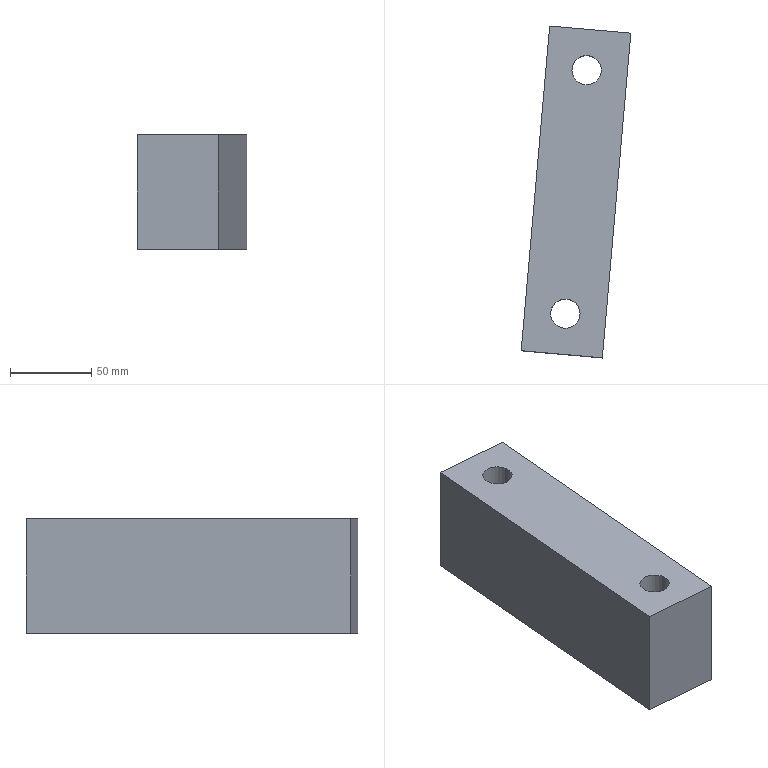Part | NX | features solid 2 | 1 solid | 8 faces | box 67.241 x 203.597 x 70 mm | volume 664374 mm3 | plane 6 | cylinder 2 | commonest cylinder face diameters 18 x2
STEP:
#1=CARTESIAN_POINT('',(193.983,-191.852,-70.));
#2=VERTEX_POINT('',#1);
#3=CARTESIAN_POINT('',(184.983,-191.852,-70.));
#4=DIRECTION('',(0.,0.,1.));
#5=DIRECTION('',(1.,0.,0.));
#6=AXIS2_PLACEMENT_3D('',#3,#4,#5);
#7=CIRCLE('',#6,9.);
#8=EDGE_CURVE('',#2,#2,#7,.T.);
#9=ORIENTED_EDGE('',*,*,#8,.F.);
#10=EDGE_LOOP('',(#9));
#11=FACE_BOUND('',#10,.T.);
#12=CARTESIAN_POINT('',(207.056,-42.423,-70.));
#13=VERTEX_POINT('',#12);
#14=CARTESIAN_POINT('',(198.056,-42.423,-70.));
#15=DIRECTION('',(0.,0.,1.));
#16=DIRECTION('',(1.,0.,0.));
#17=AXIS2_PLACEMENT_3D('',#14,#15,#16);
#18=CIRCLE('',#17,9.);
#19=EDGE_CURVE('',#13,#13,#18,.T.);
#20=ORIENTED_EDGE('',*,*,#19,.F.);
#21=EDGE_LOOP('',(#20));
#22=FACE_BOUND('',#21,.T.);
#23=CARTESIAN_POINT('',(175.33,-15.339,-70.));
#24=VERTEX_POINT('',#23);
#25=CARTESIAN_POINT('',(225.14,-19.697,-70.));
#26=VERTEX_POINT('',#25);
#27=CARTESIAN_POINT('',(175.33,-15.339,-70.));
#28=DIRECTION('',(0.9962,-0.08716,0.));
#29=VECTOR('',#28,1000.);
#30=LINE('',#27,#29);
#31=EDGE_CURVE('',#24,#26,#30,.T.);
#32=ORIENTED_EDGE('',*,*,#31,.F.);
#33=CARTESIAN_POINT('',(157.899,-214.578,-70.));
#34=VERTEX_POINT('',#33);
#35=CARTESIAN_POINT('',(162.257,-164.769,-70.));
#36=DIRECTION('',(0.08716,0.9962,0.));
#37=VECTOR('',#36,1000.);
#38=LINE('',#35,#37);
#39=EDGE_CURVE('',#34,#24,#38,.T.);
#40=ORIENTED_EDGE('',*,*,#39,.F.);
#41=CARTESIAN_POINT('',(207.709,-218.936,-70.));
#42=VERTEX_POINT('',#41);
#43=CARTESIAN_POINT('',(157.899,-214.578,-70.));
#44=DIRECTION('',(-0.9962,0.08716,0.));
#45=VECTOR('',#44,1000.);
#46=LINE('',#43,#45);
#47=EDGE_CURVE('',#34,#42,#46,.F.);
#48=ORIENTED_EDGE('',*,*,#47,.T.);
#49=CARTESIAN_POINT('',(212.067,-169.126,-70.));
#50=DIRECTION('',(-0.08716,-0.9962,0.));
#51=VECTOR('',#50,1000.);
#52=LINE('',#49,#51);
#53=EDGE_CURVE('',#42,#26,#52,.F.);
#54=ORIENTED_EDGE('',*,*,#53,.T.);
#55=EDGE_LOOP('',(#32,#40,#48,#54));
#56=FACE_BOUND('',#55,.T.);
#57=CARTESIAN_POINT('',(162.257,-164.769,-70.));
#58=DIRECTION('',(0.,0.,1.));
#59=DIRECTION('',(0.08716,0.9962,0.));
#60=AXIS2_PLACEMENT_3D('',#57,#58,#59);
#61=PLANE('',#60);
#62=ADVANCED_FACE('',(#11,#22,#56),#61,.T.);
#63=ORIENTED_EDGE('',*,*,#47,.F.);
#64=CARTESIAN_POINT('',(157.899,-214.578,-140.));
#65=VERTEX_POINT('',#64);
#66=CARTESIAN_POINT('',(157.899,-214.578,-70.));
#67=DIRECTION('',(0.,0.,1.));
#68=VECTOR('',#67,1000.);
#69=LINE('',#66,#68);
#70=EDGE_CURVE('',#34,#65,#69,.F.);
#71=ORIENTED_EDGE('',*,*,#70,.T.);
#72=CARTESIAN_POINT('',(207.709,-218.936,-140.));
#73=VERTEX_POINT('',#72);
#74=CARTESIAN_POINT('',(157.899,-214.578,-140.));
#75=DIRECTION('',(0.9962,-0.08716,0.));
#76=VECTOR('',#75,1000.);
#77=LINE('',#74,#76);
#78=EDGE_CURVE('',#65,#73,#77,.T.);
#79=ORIENTED_EDGE('',*,*,#78,.T.);
#80=CARTESIAN_POINT('',(207.709,-218.936,-70.));
#81=DIRECTION('',(0.,0.,1.));
#82=VECTOR('',#81,1000.);
#83=LINE('',#80,#82);
#84=EDGE_CURVE('',#42,#73,#83,.F.);
#85=ORIENTED_EDGE('',*,*,#84,.F.);
#86=EDGE_LOOP('',(#63,#71,#79,#85));
#87=FACE_BOUND('',#86,.T.);
#88=CARTESIAN_POINT('',(157.899,-214.578,-70.));
#89=DIRECTION('',(0.08716,0.9962,0.));
#90=DIRECTION('',(0.,0.,-1.));
#91=AXIS2_PLACEMENT_3D('',#88,#89,#90);
#92=PLANE('',#91);
#93=ADVANCED_FACE('',(#87),#92,.F.);
#94=CARTESIAN_POINT('',(193.983,-191.852,-140.));
#95=VERTEX_POINT('',#94);
#96=CARTESIAN_POINT('',(184.983,-191.852,-140.));
#97=DIRECTION('',(0.,0.,1.));
#98=DIRECTION('',(1.,0.,0.));
#99=AXIS2_PLACEMENT_3D('',#96,#97,#98);
#100=CIRCLE('',#99,9.);
#101=EDGE_CURVE('',#95,#95,#100,.F.);
#102=ORIENTED_EDGE('',*,*,#101,.F.);
#103=EDGE_LOOP('',(#102));
#104=FACE_BOUND('',#103,.T.);
#105=CARTESIAN_POINT('',(207.056,-42.423,-140.));
#106=VERTEX_POINT('',#105);
#107=CARTESIAN_POINT('',(198.056,-42.423,-140.));
#108=DIRECTION('',(0.,0.,1.));
#109=DIRECTION('',(1.,0.,0.));
#110=AXIS2_PLACEMENT_3D('',#107,#108,#109);
#111=CIRCLE('',#110,9.);
#112=EDGE_CURVE('',#106,#106,#111,.F.);
#113=ORIENTED_EDGE('',*,*,#112,.F.);
#114=EDGE_LOOP('',(#113));
#115=FACE_BOUND('',#114,.T.);
#116=ORIENTED_EDGE('',*,*,#78,.F.);
#117=CARTESIAN_POINT('',(175.33,-15.339,-140.));
#118=VERTEX_POINT('',#117);
#119=CARTESIAN_POINT('',(162.257,-164.769,-140.));
#120=DIRECTION('',(0.08716,0.9962,0.));
#121=VECTOR('',#120,1000.);
#122=LINE('',#119,#121);
#123=EDGE_CURVE('',#65,#118,#122,.T.);
#124=ORIENTED_EDGE('',*,*,#123,.T.);
#125=CARTESIAN_POINT('',(225.14,-19.697,-140.));
#126=VERTEX_POINT('',#125);
#127=CARTESIAN_POINT('',(175.33,-15.339,-140.));
#128=DIRECTION('',(0.9962,-0.08716,0.));
#129=VECTOR('',#128,1000.);
#130=LINE('',#127,#129);
#131=EDGE_CURVE('',#118,#126,#130,.T.);
#132=ORIENTED_EDGE('',*,*,#131,.T.);
#133=CARTESIAN_POINT('',(212.067,-169.126,-140.));
#134=DIRECTION('',(-0.08716,-0.9962,0.));
#135=VECTOR('',#134,1000.);
#136=LINE('',#133,#135);
#137=EDGE_CURVE('',#73,#126,#136,.F.);
#138=ORIENTED_EDGE('',*,*,#137,.F.);
#139=EDGE_LOOP('',(#116,#124,#132,#138));
#140=FACE_BOUND('',#139,.T.);
#141=CARTESIAN_POINT('',(162.257,-164.769,-140.));
#142=DIRECTION('',(0.,0.,1.));
#143=DIRECTION('',(0.08716,0.9962,0.));
#144=AXIS2_PLACEMENT_3D('',#141,#142,#143);
#145=PLANE('',#144);
#146=ADVANCED_FACE('',(#104,#115,#140),#145,.F.);
#147=ORIENTED_EDGE('',*,*,#137,.T.);
#148=CARTESIAN_POINT('',(225.14,-19.697,-70.));
#149=DIRECTION('',(0.,0.,1.));
#150=VECTOR('',#149,1000.);
#151=LINE('',#148,#150);
#152=EDGE_CURVE('',#26,#126,#151,.F.);
#153=ORIENTED_EDGE('',*,*,#152,.F.);
#154=ORIENTED_EDGE('',*,*,#53,.F.);
#155=ORIENTED_EDGE('',*,*,#84,.T.);
#156=EDGE_LOOP('',(#147,#153,#154,#155));
#157=FACE_BOUND('',#156,.T.);
#158=CARTESIAN_POINT('',(212.067,-169.126,-70.));
#159=DIRECTION('',(-0.9962,0.08716,0.));
#160=DIRECTION('',(-0.08716,-0.9962,0.));
#161=AXIS2_PLACEMENT_3D('',#158,#159,#160);
#162=PLANE('',#161);
#163=ADVANCED_FACE('',(#157),#162,.F.);
#164=CARTESIAN_POINT('',(175.33,-15.339,-70.));
#165=DIRECTION('',(0.,0.,-1.));
#166=VECTOR('',#165,1000.);
#167=LINE('',#164,#166);
#168=EDGE_CURVE('',#24,#118,#167,.T.);
#169=ORIENTED_EDGE('',*,*,#168,.F.);
#170=ORIENTED_EDGE('',*,*,#31,.T.);
#171=ORIENTED_EDGE('',*,*,#152,.T.);
#172=ORIENTED_EDGE('',*,*,#131,.F.);
#173=EDGE_LOOP('',(#169,#170,#171,#172));
#174=FACE_BOUND('',#173,.T.);
#175=CARTESIAN_POINT('',(175.33,-15.339,-70.));
#176=DIRECTION('',(0.08716,0.9962,0.));
#177=DIRECTION('',(0.,0.,-1.));
#178=AXIS2_PLACEMENT_3D('',#175,#176,#177);
#179=PLANE('',#178);
#180=ADVANCED_FACE('',(#174),#179,.T.);
#181=ORIENTED_EDGE('',*,*,#123,.F.);
#182=ORIENTED_EDGE('',*,*,#70,.F.);
#183=ORIENTED_EDGE('',*,*,#39,.T.);
#184=ORIENTED_EDGE('',*,*,#168,.T.);
#185=EDGE_LOOP('',(#181,#182,#183,#184));
#186=FACE_BOUND('',#185,.T.);
#187=CARTESIAN_POINT('',(162.257,-164.769,-70.));
#188=DIRECTION('',(-0.9962,0.08716,0.));
#189=DIRECTION('',(-0.08716,-0.9962,0.));
#190=AXIS2_PLACEMENT_3D('',#187,#188,#189);
#191=PLANE('',#190);
#192=ADVANCED_FACE('',(#186),#191,.T.);
#193=ORIENTED_EDGE('',*,*,#19,.T.);
#194=EDGE_LOOP('',(#193));
#195=FACE_BOUND('',#194,.T.);
#196=ORIENTED_EDGE('',*,*,#112,.T.);
#197=EDGE_LOOP('',(#196));
#198=FACE_BOUND('',#197,.T.);
#199=CARTESIAN_POINT('',(198.056,-42.423,-540.));
#200=DIRECTION('',(0.,0.,1.));
#201=DIRECTION('',(1.,0.,0.));
#202=AXIS2_PLACEMENT_3D('',#199,#200,#201);
#203=CYLINDRICAL_SURFACE('',#202,9.);
#204=ADVANCED_FACE('',(#195,#198),#203,.F.);
#205=ORIENTED_EDGE('',*,*,#8,.T.);
#206=EDGE_LOOP('',(#205));
#207=FACE_BOUND('',#206,.T.);
#208=ORIENTED_EDGE('',*,*,#101,.T.);
#209=EDGE_LOOP('',(#208));
#210=FACE_BOUND('',#209,.T.);
#211=CARTESIAN_POINT('',(184.983,-191.852,-540.));
#212=DIRECTION('',(0.,0.,1.));
#213=DIRECTION('',(1.,0.,0.));
#214=AXIS2_PLACEMENT_3D('',#211,#212,#213);
#215=CYLINDRICAL_SURFACE('',#214,9.);
#216=ADVANCED_FACE('',(#207,#210),#215,.F.);
#217=CLOSED_SHELL('',(#62,#93,#146,#163,#180,#192,#204,#216));
#218=MANIFOLD_SOLID_BREP('',#217);
#219=(LENGTH_UNIT()NAMED_UNIT(*)SI_UNIT(.MILLI.,.METRE.));
#220=UNCERTAINTY_MEASURE_WITH_UNIT(LENGTH_MEASURE(0.00001),#219,'','');
#221=(NAMED_UNIT(*)PLANE_ANGLE_UNIT()SI_UNIT($,.RADIAN.));
#222=(NAMED_UNIT(*)SI_UNIT($,.STERADIAN.)SOLID_ANGLE_UNIT());
#223=(GEOMETRIC_REPRESENTATION_CONTEXT(3)GLOBAL_UNCERTAINTY_ASSIGNED_CONTEXT((#220))GLOBAL_UNIT_ASSIGNED_CONTEXT((#219,#221,#222))REPRESENTATION_CONTEXT('',''));
#224=ADVANCED_BREP_SHAPE_REPRESENTATION('',(#218),#223);